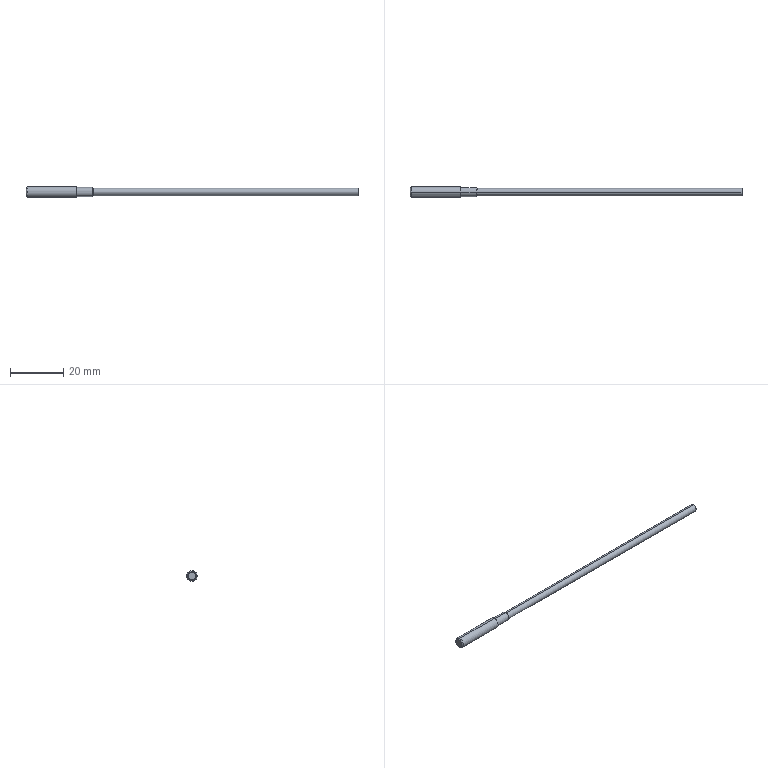Part | STEP file | C_C04_N01 | 1 solid | 20 faces | box 125 x 4.01 x 4 mm | volume 907.682 mm3 | cylinder 10 | plane 4 | cone 4 | sphere 2 | commonest cylinder face diameters 1 x2 2.8 x2 3 x2 3.4 x2 4 x2
STEP:
#1=CARTESIAN_POINT('',(0.5295,0.,2.));
#2=VERTEX_POINT('',#1);
#3=CARTESIAN_POINT('',(19.,0.,2.));
#4=VERTEX_POINT('',#3);
#5=CARTESIAN_POINT('',(0.5295,0.,2.));
#6=DIRECTION('',(1.,0.,0.));
#7=VECTOR('',#6,1000.);
#8=LINE('',#5,#7);
#9=EDGE_CURVE('',#2,#4,#8,.T.);
#10=ORIENTED_EDGE('',*,*,#9,.F.);
#11=CARTESIAN_POINT('',(0.5295,0.,-2.));
#12=VERTEX_POINT('',#11);
#13=CARTESIAN_POINT('',(0.5295,0.,0.));
#14=DIRECTION('',(1.,0.,0.));
#15=DIRECTION('',(0.,0.,-1.));
#16=AXIS2_PLACEMENT_3D('',#13,#14,#15);
#17=CIRCLE('',#16,2.);
#18=EDGE_CURVE('',#2,#12,#17,.T.);
#19=ORIENTED_EDGE('',*,*,#18,.T.);
#20=CARTESIAN_POINT('',(19.,0.,-2.));
#21=VERTEX_POINT('',#20);
#22=CARTESIAN_POINT('',(0.5295,0.,-2.));
#23=DIRECTION('',(1.,0.,0.));
#24=VECTOR('',#23,1000.);
#25=LINE('',#22,#24);
#26=EDGE_CURVE('',#12,#21,#25,.T.);
#27=ORIENTED_EDGE('',*,*,#26,.T.);
#28=CARTESIAN_POINT('',(19.,0.,0.));
#29=DIRECTION('',(1.,0.,0.));
#30=DIRECTION('',(0.,0.,-1.));
#31=AXIS2_PLACEMENT_3D('',#28,#29,#30);
#32=CIRCLE('',#31,2.);
#33=EDGE_CURVE('',#4,#21,#32,.T.);
#34=ORIENTED_EDGE('',*,*,#33,.F.);
#35=EDGE_LOOP('',(#10,#19,#27,#34));
#36=FACE_OUTER_BOUND('',#35,.T.);
#37=CARTESIAN_POINT('',(125.,0.,0.));
#38=DIRECTION('',(1.,0.,0.));
#39=DIRECTION('',(0.,1.,0.));
#40=AXIS2_PLACEMENT_3D('',#37,#38,#39);
#41=CYLINDRICAL_SURFACE('',#40,2.);
#42=ADVANCED_FACE('',(#36),#41,.T.);
#43=CARTESIAN_POINT('',(19.,0.,1.7));
#44=VERTEX_POINT('',#43);
#45=CARTESIAN_POINT('',(19.,0.,-1.7));
#46=VERTEX_POINT('',#45);
#47=CARTESIAN_POINT('',(19.,0.,0.));
#48=DIRECTION('',(1.,0.,0.));
#49=DIRECTION('',(0.,0.,-1.));
#50=AXIS2_PLACEMENT_3D('',#47,#48,#49);
#51=CIRCLE('',#50,1.7);
#52=EDGE_CURVE('',#44,#46,#51,.T.);
#53=ORIENTED_EDGE('',*,*,#52,.F.);
#54=CARTESIAN_POINT('',(19.,0.,0.));
#55=DIRECTION('',(1.,0.,0.));
#56=DIRECTION('',(0.,0.,-1.));
#57=AXIS2_PLACEMENT_3D('',#54,#55,#56);
#58=CIRCLE('',#57,1.7);
#59=EDGE_CURVE('',#46,#44,#58,.T.);
#60=ORIENTED_EDGE('',*,*,#59,.F.);
#61=EDGE_LOOP('',(#53,#60));
#62=FACE_BOUND('',#61,.T.);
#63=CARTESIAN_POINT('',(19.,0.,0.));
#64=DIRECTION('',(1.,0.,0.));
#65=DIRECTION('',(0.,0.,-1.));
#66=AXIS2_PLACEMENT_3D('',#63,#64,#65);
#67=CIRCLE('',#66,2.);
#68=EDGE_CURVE('',#21,#4,#67,.T.);
#69=ORIENTED_EDGE('',*,*,#68,.T.);
#70=ORIENTED_EDGE('',*,*,#33,.T.);
#71=EDGE_LOOP('',(#69,#70));
#72=FACE_OUTER_BOUND('',#71,.T.);
#73=CARTESIAN_POINT('',(19.,2.,0.));
#74=DIRECTION('',(-1.,0.,0.));
#75=DIRECTION('',(0.,0.,1.));
#76=AXIS2_PLACEMENT_3D('',#73,#74,#75);
#77=PLANE('',#76);
#78=ADVANCED_FACE('',(#62,#72),#77,.F.);
#79=ORIENTED_EDGE('',*,*,#9,.T.);
#80=ORIENTED_EDGE('',*,*,#68,.F.);
#81=ORIENTED_EDGE('',*,*,#26,.F.);
#82=CARTESIAN_POINT('',(0.5295,0.,0.));
#83=DIRECTION('',(1.,0.,0.));
#84=DIRECTION('',(0.,0.,-1.));
#85=AXIS2_PLACEMENT_3D('',#82,#83,#84);
#86=CIRCLE('',#85,2.);
#87=EDGE_CURVE('',#12,#2,#86,.T.);
#88=ORIENTED_EDGE('',*,*,#87,.T.);
#89=EDGE_LOOP('',(#79,#80,#81,#88));
#90=FACE_OUTER_BOUND('',#89,.T.);
#91=CARTESIAN_POINT('',(18.,1.936,0.5));
#92=VERTEX_POINT('',#91);
#93=CARTESIAN_POINT('',(18.5,2.,0.));
#94=VERTEX_POINT('',#93);
#95=CARTESIAN_POINT('',(18.,1.936,0.5));
#96=CARTESIAN_POINT('',(18.131,1.937,0.5));
#97=CARTESIAN_POINT('',(18.261,1.952,0.4459));
#98=CARTESIAN_POINT('',(18.446,1.985,0.2611));
#99=CARTESIAN_POINT('',(18.5,2.,0.1308));
#100=CARTESIAN_POINT('',(18.5,2.,0.));
#101=B_SPLINE_CURVE_WITH_KNOTS('',3,(#95,#96,#97,#98,#99,#100),.UNSPECIFIED.,.F.,.F.,(4,2,4),(0.75,0.875,1.),.UNSPECIFIED.);
#102=EDGE_CURVE('',#92,#94,#101,.T.);
#103=ORIENTED_EDGE('',*,*,#102,.F.);
#104=CARTESIAN_POINT('',(18.,1.936,-0.5));
#105=VERTEX_POINT('',#104);
#106=CARTESIAN_POINT('',(18.,1.936,-0.5));
#107=CARTESIAN_POINT('',(17.868,1.937,-0.5));
#108=CARTESIAN_POINT('',(17.739,1.952,-0.4456));
#109=CARTESIAN_POINT('',(17.555,1.985,-0.2617));
#110=CARTESIAN_POINT('',(17.5,2.,-0.1318));
#111=CARTESIAN_POINT('',(17.5,2.,0.1317));
#112=CARTESIAN_POINT('',(17.554,1.985,0.2614));
#113=CARTESIAN_POINT('',(17.739,1.952,0.4458));
#114=CARTESIAN_POINT('',(17.869,1.937,0.5));
#115=CARTESIAN_POINT('',(18.,1.936,0.5));
#116=B_SPLINE_CURVE_WITH_KNOTS('',3,(#106,#107,#108,#109,#110,#111,#112,#113,#114,#115),.UNSPECIFIED.,.F.,.F.,(4,2,2,2,4),(0.25,0.375,0.5,0.625,0.75),.UNSPECIFIED.);
#117=EDGE_CURVE('',#105,#92,#116,.T.);
#118=ORIENTED_EDGE('',*,*,#117,.F.);
#119=CARTESIAN_POINT('',(18.5,2.,0.));
#120=CARTESIAN_POINT('',(18.5,2.,-0.1308));
#121=CARTESIAN_POINT('',(18.446,1.985,-0.2611));
#122=CARTESIAN_POINT('',(18.261,1.952,-0.4458));
#123=CARTESIAN_POINT('',(18.132,1.937,-0.5));
#124=CARTESIAN_POINT('',(18.,1.936,-0.5));
#125=B_SPLINE_CURVE_WITH_KNOTS('',3,(#119,#120,#121,#122,#123,#124),.UNSPECIFIED.,.F.,.F.,(4,2,4),(0.,0.125,0.25),.UNSPECIFIED.);
#126=EDGE_CURVE('',#94,#105,#125,.T.);
#127=ORIENTED_EDGE('',*,*,#126,.F.);
#128=EDGE_LOOP('',(#103,#118,#127));
#129=FACE_BOUND('',#128,.T.);
#130=CARTESIAN_POINT('',(125.,0.,0.));
#131=DIRECTION('',(1.,0.,0.));
#132=DIRECTION('',(0.,-1.,0.));
#133=AXIS2_PLACEMENT_3D('',#130,#131,#132);
#134=CYLINDRICAL_SURFACE('',#133,2.);
#135=ADVANCED_FACE('',(#90,#129),#134,.T.);
#136=CARTESIAN_POINT('',(18.,1.6,0.5));
#137=VERTEX_POINT('',#136);
#138=CARTESIAN_POINT('',(18.,1.936,0.5));
#139=DIRECTION('',(0.,-1.,0.));
#140=VECTOR('',#139,1000.);
#141=LINE('',#138,#140);
#142=EDGE_CURVE('',#92,#137,#141,.T.);
#143=ORIENTED_EDGE('',*,*,#142,.F.);
#144=ORIENTED_EDGE('',*,*,#102,.T.);
#145=ORIENTED_EDGE('',*,*,#126,.T.);
#146=CARTESIAN_POINT('',(18.,1.6,-0.5));
#147=VERTEX_POINT('',#146);
#148=CARTESIAN_POINT('',(18.,1.936,-0.5));
#149=DIRECTION('',(0.,-1.,0.));
#150=VECTOR('',#149,1000.);
#151=LINE('',#148,#150);
#152=EDGE_CURVE('',#105,#147,#151,.T.);
#153=ORIENTED_EDGE('',*,*,#152,.T.);
#154=CARTESIAN_POINT('',(18.5,1.6,0.));
#155=VERTEX_POINT('',#154);
#156=CARTESIAN_POINT('',(18.5,1.6,0.));
#157=CARTESIAN_POINT('',(18.5,1.6,-0.1309));
#158=CARTESIAN_POINT('',(18.446,1.6,-0.261));
#159=CARTESIAN_POINT('',(18.261,1.6,-0.4461));
#160=CARTESIAN_POINT('',(18.131,1.6,-0.5));
#161=CARTESIAN_POINT('',(18.,1.6,-0.5));
#162=B_SPLINE_CURVE_WITH_KNOTS('',3,(#156,#157,#158,#159,#160,#161),.UNSPECIFIED.,.F.,.F.,(4,2,4),(0.,0.7854,1.571),.UNSPECIFIED.);
#163=EDGE_CURVE('',#155,#147,#162,.T.);
#164=ORIENTED_EDGE('',*,*,#163,.F.);
#165=CARTESIAN_POINT('',(18.,1.6,0.5));
#166=CARTESIAN_POINT('',(18.131,1.6,0.5));
#167=CARTESIAN_POINT('',(18.261,1.6,0.4461));
#168=CARTESIAN_POINT('',(18.446,1.6,0.261));
#169=CARTESIAN_POINT('',(18.5,1.6,0.1309));
#170=CARTESIAN_POINT('',(18.5,1.6,0.));
#171=B_SPLINE_CURVE_WITH_KNOTS('',3,(#165,#166,#167,#168,#169,#170),.UNSPECIFIED.,.F.,.F.,(4,2,4),(0.,0.7854,1.571),.UNSPECIFIED.);
#172=EDGE_CURVE('',#137,#155,#171,.T.);
#173=ORIENTED_EDGE('',*,*,#172,.F.);
#174=EDGE_LOOP('',(#143,#144,#145,#153,#164,#173));
#175=FACE_OUTER_BOUND('',#174,.T.);
#176=CARTESIAN_POINT('',(18.,1.5,0.));
#177=DIRECTION('',(0.,-1.,0.));
#178=DIRECTION('',(-1.,0.,0.));
#179=AXIS2_PLACEMENT_3D('',#176,#177,#178);
#180=CYLINDRICAL_SURFACE('',#179,0.5);
#181=ADVANCED_FACE('',(#175),#180,.F.);
#182=CARTESIAN_POINT('',(17.5,1.6,0.));
#183=VERTEX_POINT('',#182);
#184=CARTESIAN_POINT('',(18.,1.5,0.));
#185=DIRECTION('',(0.,0.,-1.));
#186=DIRECTION('',(-0.9804,0.1971,0.));
#187=AXIS2_PLACEMENT_3D('',#184,#185,#186);
#188=CIRCLE('',#187,0.51);
#189=EDGE_CURVE('',#183,#155,#188,.T.);
#190=ORIENTED_EDGE('',*,*,#189,.F.);
#191=CARTESIAN_POINT('',(17.5,1.6,0.));
#192=CARTESIAN_POINT('',(17.5,1.6,0.1309));
#193=CARTESIAN_POINT('',(17.554,1.6,0.261));
#194=CARTESIAN_POINT('',(17.739,1.6,0.4461));
#195=CARTESIAN_POINT('',(17.869,1.6,0.5));
#196=CARTESIAN_POINT('',(18.,1.6,0.5));
#197=B_SPLINE_CURVE_WITH_KNOTS('',3,(#191,#192,#193,#194,#195,#196),.UNSPECIFIED.,.F.,.F.,(4,2,4),(0.,0.7854,1.571),.UNSPECIFIED.);
#198=EDGE_CURVE('',#183,#137,#197,.T.);
#199=ORIENTED_EDGE('',*,*,#198,.T.);
#200=ORIENTED_EDGE('',*,*,#172,.T.);
#201=EDGE_LOOP('',(#190,#199,#200));
#202=FACE_OUTER_BOUND('',#201,.T.);
#203=CARTESIAN_POINT('',(18.,1.5,0.));
#204=DIRECTION('',(1.,0.,0.));
#205=DIRECTION('',(0.,0.,-1.));
#206=AXIS2_PLACEMENT_3D('',#203,#204,#205);
#207=SPHERICAL_SURFACE('',#206,0.51);
#208=ADVANCED_FACE('',(#202),#207,.T.);
#209=ORIENTED_EDGE('',*,*,#189,.T.);
#210=ORIENTED_EDGE('',*,*,#163,.T.);
#211=CARTESIAN_POINT('',(18.,1.6,-0.5));
#212=CARTESIAN_POINT('',(17.869,1.6,-0.5));
#213=CARTESIAN_POINT('',(17.739,1.6,-0.4461));
#214=CARTESIAN_POINT('',(17.554,1.6,-0.261));
#215=CARTESIAN_POINT('',(17.5,1.6,-0.1309));
#216=CARTESIAN_POINT('',(17.5,1.6,0.));
#217=B_SPLINE_CURVE_WITH_KNOTS('',3,(#211,#212,#213,#214,#215,#216),.UNSPECIFIED.,.F.,.F.,(4,2,4),(0.,0.7854,1.571),.UNSPECIFIED.);
#218=EDGE_CURVE('',#147,#183,#217,.T.);
#219=ORIENTED_EDGE('',*,*,#218,.T.);
#220=EDGE_LOOP('',(#209,#210,#219));
#221=FACE_OUTER_BOUND('',#220,.T.);
#222=CARTESIAN_POINT('',(18.,1.5,0.));
#223=DIRECTION('',(-1.,0.,0.));
#224=DIRECTION('',(0.,0.,1.));
#225=AXIS2_PLACEMENT_3D('',#222,#223,#224);
#226=SPHERICAL_SURFACE('',#225,0.51);
#227=ADVANCED_FACE('',(#221),#226,.T.);
#228=ORIENTED_EDGE('',*,*,#142,.T.);
#229=ORIENTED_EDGE('',*,*,#198,.F.);
#230=ORIENTED_EDGE('',*,*,#218,.F.);
#231=ORIENTED_EDGE('',*,*,#152,.F.);
#232=ORIENTED_EDGE('',*,*,#117,.T.);
#233=EDGE_LOOP('',(#228,#229,#230,#231,#232));
#234=FACE_OUTER_BOUND('',#233,.T.);
#235=CARTESIAN_POINT('',(18.,1.5,0.));
#236=DIRECTION('',(0.,-1.,0.));
#237=DIRECTION('',(1.,0.,0.));
#238=AXIS2_PLACEMENT_3D('',#235,#236,#237);
#239=CYLINDRICAL_SURFACE('',#238,0.5);
#240=ADVANCED_FACE('',(#234),#239,.F.);
#241=CARTESIAN_POINT('',(0.1,0.,1.571));
#242=VERTEX_POINT('',#241);
#243=CARTESIAN_POINT('',(0.1,0.,1.571));
#244=DIRECTION('',(0.7071,0.,0.7071));
#245=VECTOR('',#244,1000.);
#246=LINE('',#243,#245);
#247=EDGE_CURVE('',#242,#2,#246,.T.);
#248=ORIENTED_EDGE('',*,*,#247,.T.);
#249=ORIENTED_EDGE('',*,*,#87,.F.);
#250=CARTESIAN_POINT('',(0.1,0.,-1.571));
#251=VERTEX_POINT('',#250);
#252=CARTESIAN_POINT('',(0.1,0.,-1.571));
#253=DIRECTION('',(0.7071,0.,-0.7071));
#254=VECTOR('',#253,1000.);
#255=LINE('',#252,#254);
#256=EDGE_CURVE('',#251,#12,#255,.T.);
#257=ORIENTED_EDGE('',*,*,#256,.F.);
#258=CARTESIAN_POINT('',(0.1,0.,0.));
#259=DIRECTION('',(1.,0.,0.));
#260=DIRECTION('',(0.,0.,-1.));
#261=AXIS2_PLACEMENT_3D('',#258,#259,#260);
#262=CIRCLE('',#261,1.571);
#263=EDGE_CURVE('',#251,#242,#262,.T.);
#264=ORIENTED_EDGE('',*,*,#263,.T.);
#265=EDGE_LOOP('',(#248,#249,#257,#264));
#266=FACE_OUTER_BOUND('',#265,.T.);
#267=CARTESIAN_POINT('',(0.1,0.,0.));
#268=DIRECTION('',(1.,0.,0.));
#269=DIRECTION('',(0.,-1.,0.));
#270=AXIS2_PLACEMENT_3D('',#267,#268,#269);
#271=CONICAL_SURFACE('',#270,1.571,0.7854);
#272=ADVANCED_FACE('',(#266),#271,.T.);
#273=CARTESIAN_POINT('',(0.1,0.,0.));
#274=DIRECTION('',(1.,0.,0.));
#275=DIRECTION('',(0.,0.,-1.));
#276=AXIS2_PLACEMENT_3D('',#273,#274,#275);
#277=CIRCLE('',#276,1.571);
#278=EDGE_CURVE('',#242,#251,#277,.T.);
#279=ORIENTED_EDGE('',*,*,#278,.F.);
#280=ORIENTED_EDGE('',*,*,#263,.F.);
#281=EDGE_LOOP('',(#279,#280));
#282=FACE_OUTER_BOUND('',#281,.T.);
#283=CARTESIAN_POINT('',(0.1,0.,-1.5));
#284=VERTEX_POINT('',#283);
#285=CARTESIAN_POINT('',(0.1,0.,1.5));
#286=VERTEX_POINT('',#285);
#287=CARTESIAN_POINT('',(0.1,0.,0.));
#288=DIRECTION('',(1.,0.,0.));
#289=DIRECTION('',(0.,0.,-1.));
#290=AXIS2_PLACEMENT_3D('',#287,#288,#289);
#291=CIRCLE('',#290,1.5);
#292=EDGE_CURVE('',#284,#286,#291,.T.);
#293=ORIENTED_EDGE('',*,*,#292,.T.);
#294=CARTESIAN_POINT('',(0.1,0.,0.));
#295=DIRECTION('',(1.,0.,0.));
#296=DIRECTION('',(0.,0.,-1.));
#297=AXIS2_PLACEMENT_3D('',#294,#295,#296);
#298=CIRCLE('',#297,1.5);
#299=EDGE_CURVE('',#286,#284,#298,.T.);
#300=ORIENTED_EDGE('',*,*,#299,.T.);
#301=EDGE_LOOP('',(#293,#300));
#302=FACE_BOUND('',#301,.T.);
#303=CARTESIAN_POINT('',(0.1,1.5,0.));
#304=DIRECTION('',(1.,0.,0.));
#305=DIRECTION('',(0.,0.,-1.));
#306=AXIS2_PLACEMENT_3D('',#303,#304,#305);
#307=PLANE('',#306);
#308=ADVANCED_FACE('',(#282,#302),#307,.F.);
#309=CARTESIAN_POINT('',(0.,0.,1.5));
#310=VERTEX_POINT('',#309);
#311=CARTESIAN_POINT('',(0.,0.,1.5));
#312=DIRECTION('',(1.,0.,0.));
#313=VECTOR('',#312,1000.);
#314=LINE('',#311,#313);
#315=EDGE_CURVE('',#310,#286,#314,.T.);
#316=ORIENTED_EDGE('',*,*,#315,.F.);
#317=CARTESIAN_POINT('',(0.,0.,-1.5));
#318=VERTEX_POINT('',#317);
#319=CARTESIAN_POINT('',(0.,0.,0.));
#320=DIRECTION('',(1.,0.,0.));
#321=DIRECTION('',(0.,0.,-1.));
#322=AXIS2_PLACEMENT_3D('',#319,#320,#321);
#323=CIRCLE('',#322,1.5);
#324=EDGE_CURVE('',#310,#318,#323,.T.);
#325=ORIENTED_EDGE('',*,*,#324,.T.);
#326=CARTESIAN_POINT('',(0.,0.,-1.5));
#327=DIRECTION('',(1.,0.,0.));
#328=VECTOR('',#327,1000.);
#329=LINE('',#326,#328);
#330=EDGE_CURVE('',#318,#284,#329,.T.);
#331=ORIENTED_EDGE('',*,*,#330,.T.);
#332=ORIENTED_EDGE('',*,*,#299,.F.);
#333=EDGE_LOOP('',(#316,#325,#331,#332));
#334=FACE_OUTER_BOUND('',#333,.T.);
#335=CARTESIAN_POINT('',(125.,0.,0.));
#336=DIRECTION('',(1.,0.,0.));
#337=DIRECTION('',(0.,1.,0.));
#338=AXIS2_PLACEMENT_3D('',#335,#336,#337);
#339=CYLINDRICAL_SURFACE('',#338,1.5);
#340=ADVANCED_FACE('',(#334),#339,.T.);
#341=ORIENTED_EDGE('',*,*,#315,.T.);
#342=ORIENTED_EDGE('',*,*,#292,.F.);
#343=ORIENTED_EDGE('',*,*,#330,.F.);
#344=CARTESIAN_POINT('',(0.,0.,0.));
#345=DIRECTION('',(1.,0.,0.));
#346=DIRECTION('',(0.,0.,-1.));
#347=AXIS2_PLACEMENT_3D('',#344,#345,#346);
#348=CIRCLE('',#347,1.5);
#349=EDGE_CURVE('',#318,#310,#348,.T.);
#350=ORIENTED_EDGE('',*,*,#349,.T.);
#351=EDGE_LOOP('',(#341,#342,#343,#350));
#352=FACE_OUTER_BOUND('',#351,.T.);
#353=CARTESIAN_POINT('',(125.,0.,0.));
#354=DIRECTION('',(1.,0.,0.));
#355=DIRECTION('',(0.,-1.,0.));
#356=AXIS2_PLACEMENT_3D('',#353,#354,#355);
#357=CYLINDRICAL_SURFACE('',#356,1.5);
#358=ADVANCED_FACE('',(#352),#357,.T.);
#359=ORIENTED_EDGE('',*,*,#324,.F.);
#360=ORIENTED_EDGE('',*,*,#349,.F.);
#361=EDGE_LOOP('',(#359,#360));
#362=FACE_OUTER_BOUND('',#361,.T.);
#363=CARTESIAN_POINT('',(0.,0.,0.));
#364=DIRECTION('',(1.,0.,0.));
#365=DIRECTION('',(0.,0.,-1.));
#366=AXIS2_PLACEMENT_3D('',#363,#364,#365);
#367=PLANE('',#366);
#368=ADVANCED_FACE('',(#362),#367,.F.);
#369=ORIENTED_EDGE('',*,*,#247,.F.);
#370=ORIENTED_EDGE('',*,*,#278,.T.);
#371=ORIENTED_EDGE('',*,*,#256,.T.);
#372=ORIENTED_EDGE('',*,*,#18,.F.);
#373=EDGE_LOOP('',(#369,#370,#371,#372));
#374=FACE_OUTER_BOUND('',#373,.T.);
#375=CARTESIAN_POINT('',(0.1,0.,0.));
#376=DIRECTION('',(1.,0.,0.));
#377=DIRECTION('',(0.,1.,0.));
#378=AXIS2_PLACEMENT_3D('',#375,#376,#377);
#379=CONICAL_SURFACE('',#378,1.571,0.7854);
#380=ADVANCED_FACE('',(#374),#379,.T.);
#381=CARTESIAN_POINT('',(25.,0.,1.7));
#382=VERTEX_POINT('',#381);
#383=CARTESIAN_POINT('',(19.,0.,1.7));
#384=DIRECTION('',(1.,0.,0.));
#385=VECTOR('',#384,1000.);
#386=LINE('',#383,#385);
#387=EDGE_CURVE('',#44,#382,#386,.T.);
#388=ORIENTED_EDGE('',*,*,#387,.T.);
#389=CARTESIAN_POINT('',(25.,0.,-1.7));
#390=VERTEX_POINT('',#389);
#391=CARTESIAN_POINT('',(25.,0.,0.));
#392=DIRECTION('',(1.,0.,0.));
#393=DIRECTION('',(0.,0.,-1.));
#394=AXIS2_PLACEMENT_3D('',#391,#392,#393);
#395=CIRCLE('',#394,1.7);
#396=EDGE_CURVE('',#390,#382,#395,.T.);
#397=ORIENTED_EDGE('',*,*,#396,.F.);
#398=CARTESIAN_POINT('',(19.,0.,-1.7));
#399=DIRECTION('',(1.,0.,0.));
#400=VECTOR('',#399,1000.);
#401=LINE('',#398,#400);
#402=EDGE_CURVE('',#46,#390,#401,.T.);
#403=ORIENTED_EDGE('',*,*,#402,.F.);
#404=ORIENTED_EDGE('',*,*,#59,.T.);
#405=EDGE_LOOP('',(#388,#397,#403,#404));
#406=FACE_OUTER_BOUND('',#405,.T.);
#407=CARTESIAN_POINT('',(125.,0.,0.));
#408=DIRECTION('',(1.,0.,0.));
#409=DIRECTION('',(0.,-1.,0.));
#410=AXIS2_PLACEMENT_3D('',#407,#408,#409);
#411=CYLINDRICAL_SURFACE('',#410,1.7);
#412=ADVANCED_FACE('',(#406),#411,.T.);
#413=ORIENTED_EDGE('',*,*,#387,.F.);
#414=ORIENTED_EDGE('',*,*,#52,.T.);
#415=ORIENTED_EDGE('',*,*,#402,.T.);
#416=CARTESIAN_POINT('',(25.,0.,0.));
#417=DIRECTION('',(1.,0.,0.));
#418=DIRECTION('',(0.,0.,-1.));
#419=AXIS2_PLACEMENT_3D('',#416,#417,#418);
#420=CIRCLE('',#419,1.7);
#421=EDGE_CURVE('',#382,#390,#420,.T.);
#422=ORIENTED_EDGE('',*,*,#421,.F.);
#423=EDGE_LOOP('',(#413,#414,#415,#422));
#424=FACE_OUTER_BOUND('',#423,.T.);
#425=CARTESIAN_POINT('',(125.,0.,0.));
#426=DIRECTION('',(1.,0.,0.));
#427=DIRECTION('',(0.,1.,0.));
#428=AXIS2_PLACEMENT_3D('',#425,#426,#427);
#429=CYLINDRICAL_SURFACE('',#428,1.7);
#430=ADVANCED_FACE('',(#424),#429,.T.);
#431=CARTESIAN_POINT('',(25.3,0.,-1.4));
#432=VERTEX_POINT('',#431);
#433=CARTESIAN_POINT('',(25.3,0.,-1.4));
#434=DIRECTION('',(-0.7071,0.,-0.7071));
#435=VECTOR('',#434,1000.);
#436=LINE('',#433,#435);
#437=EDGE_CURVE('',#432,#390,#436,.T.);
#438=ORIENTED_EDGE('',*,*,#437,.F.);
#439=CARTESIAN_POINT('',(25.3,0.,1.4));
#440=VERTEX_POINT('',#439);
#441=CARTESIAN_POINT('',(25.3,0.,0.));
#442=DIRECTION('',(1.,0.,0.));
#443=DIRECTION('',(0.,0.,-1.));
#444=AXIS2_PLACEMENT_3D('',#441,#442,#443);
#445=CIRCLE('',#444,1.4);
#446=EDGE_CURVE('',#440,#432,#445,.T.);
#447=ORIENTED_EDGE('',*,*,#446,.F.);
#448=CARTESIAN_POINT('',(25.3,0.,1.4));
#449=DIRECTION('',(-0.7071,0.,0.7071));
#450=VECTOR('',#449,1000.);
#451=LINE('',#448,#450);
#452=EDGE_CURVE('',#440,#382,#451,.T.);
#453=ORIENTED_EDGE('',*,*,#452,.T.);
#454=ORIENTED_EDGE('',*,*,#421,.T.);
#455=EDGE_LOOP('',(#438,#447,#453,#454));
#456=FACE_OUTER_BOUND('',#455,.T.);
#457=CARTESIAN_POINT('',(25.,0.,0.));
#458=DIRECTION('',(-1.,0.,0.));
#459=DIRECTION('',(0.,1.,0.));
#460=AXIS2_PLACEMENT_3D('',#457,#458,#459);
#461=CONICAL_SURFACE('',#460,1.7,0.7854);
#462=ADVANCED_FACE('',(#456),#461,.T.);
#463=ORIENTED_EDGE('',*,*,#437,.T.);
#464=ORIENTED_EDGE('',*,*,#396,.T.);
#465=ORIENTED_EDGE('',*,*,#452,.F.);
#466=CARTESIAN_POINT('',(25.3,0.,0.));
#467=DIRECTION('',(1.,0.,0.));
#468=DIRECTION('',(0.,0.,-1.));
#469=AXIS2_PLACEMENT_3D('',#466,#467,#468);
#470=CIRCLE('',#469,1.4);
#471=EDGE_CURVE('',#432,#440,#470,.T.);
#472=ORIENTED_EDGE('',*,*,#471,.F.);
#473=EDGE_LOOP('',(#463,#464,#465,#472));
#474=FACE_OUTER_BOUND('',#473,.T.);
#475=CARTESIAN_POINT('',(25.,0.,0.));
#476=DIRECTION('',(-1.,0.,0.));
#477=DIRECTION('',(0.,-1.,0.));
#478=AXIS2_PLACEMENT_3D('',#475,#476,#477);
#479=CONICAL_SURFACE('',#478,1.7,0.7854);
#480=ADVANCED_FACE('',(#474),#479,.T.);
#481=CARTESIAN_POINT('',(125.,0.,1.4));
#482=VERTEX_POINT('',#481);
#483=CARTESIAN_POINT('',(25.3,0.,1.4));
#484=DIRECTION('',(1.,0.,0.));
#485=VECTOR('',#484,1000.);
#486=LINE('',#483,#485);
#487=EDGE_CURVE('',#440,#482,#486,.T.);
#488=ORIENTED_EDGE('',*,*,#487,.T.);
#489=CARTESIAN_POINT('',(125.,0.,-1.4));
#490=VERTEX_POINT('',#489);
#491=CARTESIAN_POINT('',(125.,0.,0.));
#492=DIRECTION('',(1.,0.,0.));
#493=DIRECTION('',(0.,0.,-1.));
#494=AXIS2_PLACEMENT_3D('',#491,#492,#493);
#495=CIRCLE('',#494,1.4);
#496=EDGE_CURVE('',#490,#482,#495,.T.);
#497=ORIENTED_EDGE('',*,*,#496,.F.);
#498=CARTESIAN_POINT('',(25.3,0.,-1.4));
#499=DIRECTION('',(1.,0.,0.));
#500=VECTOR('',#499,1000.);
#501=LINE('',#498,#500);
#502=EDGE_CURVE('',#432,#490,#501,.T.);
#503=ORIENTED_EDGE('',*,*,#502,.F.);
#504=ORIENTED_EDGE('',*,*,#471,.T.);
#505=EDGE_LOOP('',(#488,#497,#503,#504));
#506=FACE_OUTER_BOUND('',#505,.T.);
#507=CARTESIAN_POINT('',(125.,0.,0.));
#508=DIRECTION('',(1.,0.,0.));
#509=DIRECTION('',(0.,-1.,0.));
#510=AXIS2_PLACEMENT_3D('',#507,#508,#509);
#511=CYLINDRICAL_SURFACE('',#510,1.4);
#512=ADVANCED_FACE('',(#506),#511,.T.);
#513=ORIENTED_EDGE('',*,*,#487,.F.);
#514=ORIENTED_EDGE('',*,*,#446,.T.);
#515=ORIENTED_EDGE('',*,*,#502,.T.);
#516=CARTESIAN_POINT('',(125.,0.,0.));
#517=DIRECTION('',(1.,0.,0.));
#518=DIRECTION('',(0.,0.,-1.));
#519=AXIS2_PLACEMENT_3D('',#516,#517,#518);
#520=CIRCLE('',#519,1.4);
#521=EDGE_CURVE('',#482,#490,#520,.T.);
#522=ORIENTED_EDGE('',*,*,#521,.F.);
#523=EDGE_LOOP('',(#513,#514,#515,#522));
#524=FACE_OUTER_BOUND('',#523,.T.);
#525=CARTESIAN_POINT('',(125.,0.,0.));
#526=DIRECTION('',(1.,0.,0.));
#527=DIRECTION('',(0.,1.,0.));
#528=AXIS2_PLACEMENT_3D('',#525,#526,#527);
#529=CYLINDRICAL_SURFACE('',#528,1.4);
#530=ADVANCED_FACE('',(#524),#529,.T.);
#531=ORIENTED_EDGE('',*,*,#496,.T.);
#532=ORIENTED_EDGE('',*,*,#521,.T.);
#533=EDGE_LOOP('',(#531,#532));
#534=FACE_OUTER_BOUND('',#533,.T.);
#535=CARTESIAN_POINT('',(125.,1.4,0.));
#536=DIRECTION('',(-1.,0.,0.));
#537=DIRECTION('',(0.,0.,1.));
#538=AXIS2_PLACEMENT_3D('',#535,#536,#537);
#539=PLANE('',#538);
#540=ADVANCED_FACE('',(#534),#539,.F.);
#541=CLOSED_SHELL('',(#42,#78,#135,#181,#208,#227,#240,#272,#308,#340,#358,#368,#380,#412,#430,#462,#480,#512,#530,#540));
#542=MANIFOLD_SOLID_BREP('',#541);
#543=CARTESIAN_POINT('',(0.,0.,0.));
#544=DIRECTION('',(0.,0.,1.));
#545=DIRECTION('',(1.,0.,0.));
#546=AXIS2_PLACEMENT_3D('',#543,#544,#545);
#547=(LENGTH_UNIT()NAMED_UNIT(*)SI_UNIT(.MILLI.,.METRE.));
#548=UNCERTAINTY_MEASURE_WITH_UNIT(LENGTH_MEASURE(0.00001),#547,'','');
#549=(NAMED_UNIT(*)PLANE_ANGLE_UNIT()SI_UNIT($,.RADIAN.));
#550=(NAMED_UNIT(*)SI_UNIT($,.STERADIAN.)SOLID_ANGLE_UNIT());
#551=(GEOMETRIC_REPRESENTATION_CONTEXT(3)GLOBAL_UNCERTAINTY_ASSIGNED_CONTEXT((#548))GLOBAL_UNIT_ASSIGNED_CONTEXT((#547,#549,#550))REPRESENTATION_CONTEXT('',''));
#552=ADVANCED_BREP_SHAPE_REPRESENTATION('',(#542,#546),#551);